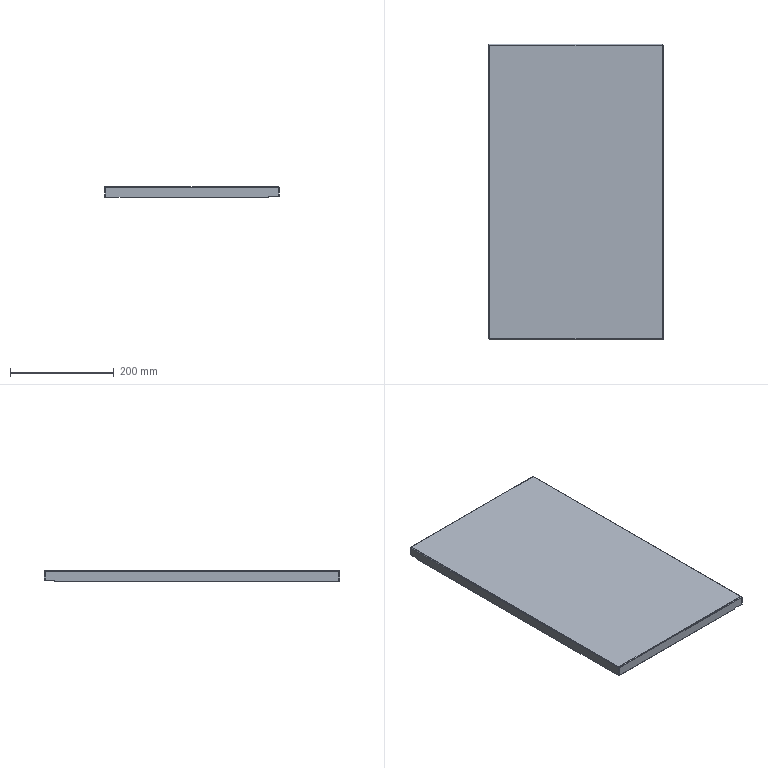Part | SolidWorks | features BaseBody 1 | 1 solid | 44 faces | box 336 x 570 x 20 mm | volume 267174 mm3 | plane 32 | cylinder 8 | spline 4 | commonest cylinder face diameters 1 x4 3.4 x4
STEP:
#1=CARTESIAN_POINT('',(-168.,265.3,-20.));
#2=VERTEX_POINT('',#1);
#3=CARTESIAN_POINT('',(-168.,265.3,-18.));
#4=VERTEX_POINT('',#3);
#5=CARTESIAN_POINT('',(-168.,265.3,-20.));
#6=DIRECTION('',(0.,0.,1.));
#7=VECTOR('',#6,1000.);
#8=LINE('',#5,#7);
#9=EDGE_CURVE('',#2,#4,#8,.T.);
#10=ORIENTED_EDGE('',*,*,#9,.T.);
#11=CARTESIAN_POINT('',(-166.8,265.3,-18.));
#12=VERTEX_POINT('',#11);
#13=CARTESIAN_POINT('',(-166.8,265.3,-18.));
#14=DIRECTION('',(-1.,0.,0.));
#15=VECTOR('',#14,1000.);
#16=LINE('',#13,#15);
#17=EDGE_CURVE('',#12,#4,#16,.T.);
#18=ORIENTED_EDGE('',*,*,#17,.F.);
#19=CARTESIAN_POINT('',(-166.8,265.3,-20.));
#20=VERTEX_POINT('',#19);
#21=CARTESIAN_POINT('',(-166.8,265.3,-20.));
#22=DIRECTION('',(0.,0.,1.));
#23=VECTOR('',#22,1000.);
#24=LINE('',#21,#23);
#25=EDGE_CURVE('',#20,#12,#24,.T.);
#26=ORIENTED_EDGE('',*,*,#25,.F.);
#27=CARTESIAN_POINT('',(-166.8,265.3,-20.));
#28=DIRECTION('',(-1.,0.,0.));
#29=VECTOR('',#28,1000.);
#30=LINE('',#27,#29);
#31=EDGE_CURVE('',#20,#2,#30,.T.);
#32=ORIENTED_EDGE('',*,*,#31,.T.);
#33=EDGE_LOOP('',(#10,#18,#26,#32));
#34=FACE_OUTER_BOUND('',#33,.T.);
#35=CARTESIAN_POINT('',(-166.8,265.3,-20.));
#36=DIRECTION('',(0.,-1.,0.));
#37=DIRECTION('',(0.,0.,-1.));
#38=AXIS2_PLACEMENT_3D('',#35,#36,#37);
#39=PLANE('',#38);
#40=ADVANCED_FACE('',(#34),#39,.F.);
#41=CARTESIAN_POINT('',(-168.,283.3,-18.));
#42=VERTEX_POINT('',#41);
#43=CARTESIAN_POINT('',(-168.,283.3,-18.));
#44=DIRECTION('',(0.,1.,0.));
#45=VECTOR('',#44,1000.);
#46=LINE('',#43,#45);
#47=EDGE_CURVE('',#4,#42,#46,.T.);
#48=ORIENTED_EDGE('',*,*,#47,.T.);
#49=CARTESIAN_POINT('',(-166.8,283.3,-18.));
#50=VERTEX_POINT('',#49);
#51=CARTESIAN_POINT('',(-166.8,283.3,-18.));
#52=DIRECTION('',(-1.,0.,0.));
#53=VECTOR('',#52,1000.);
#54=LINE('',#51,#53);
#55=EDGE_CURVE('',#50,#42,#54,.T.);
#56=ORIENTED_EDGE('',*,*,#55,.F.);
#57=CARTESIAN_POINT('',(-166.8,283.3,-18.));
#58=DIRECTION('',(0.,1.,0.));
#59=VECTOR('',#58,1000.);
#60=LINE('',#57,#59);
#61=EDGE_CURVE('',#12,#50,#60,.T.);
#62=ORIENTED_EDGE('',*,*,#61,.F.);
#63=ORIENTED_EDGE('',*,*,#17,.T.);
#64=EDGE_LOOP('',(#48,#56,#62,#63));
#65=FACE_OUTER_BOUND('',#64,.T.);
#66=CARTESIAN_POINT('',(-166.8,283.3,-18.));
#67=DIRECTION('',(0.,0.,1.));
#68=DIRECTION('',(1.,0.,0.));
#69=AXIS2_PLACEMENT_3D('',#66,#67,#68);
#70=PLANE('',#69);
#71=ADVANCED_FACE('',(#65),#70,.F.);
#72=CARTESIAN_POINT('',(166.3,-285.,-18.));
#73=VERTEX_POINT('',#72);
#74=CARTESIAN_POINT('',(148.3,-285.,-18.));
#75=VERTEX_POINT('',#74);
#76=CARTESIAN_POINT('',(166.3,-285.,-18.));
#77=DIRECTION('',(-1.,0.,0.));
#78=VECTOR('',#77,1000.);
#79=LINE('',#76,#78);
#80=EDGE_CURVE('',#73,#75,#79,.T.);
#81=ORIENTED_EDGE('',*,*,#80,.T.);
#82=CARTESIAN_POINT('',(148.3,-283.8,-18.));
#83=VERTEX_POINT('',#82);
#84=CARTESIAN_POINT('',(148.3,-283.8,-18.));
#85=DIRECTION('',(0.,-1.,0.));
#86=VECTOR('',#85,1000.);
#87=LINE('',#84,#86);
#88=EDGE_CURVE('',#83,#75,#87,.T.);
#89=ORIENTED_EDGE('',*,*,#88,.F.);
#90=CARTESIAN_POINT('',(166.3,-283.8,-18.));
#91=VERTEX_POINT('',#90);
#92=CARTESIAN_POINT('',(166.3,-283.8,-18.));
#93=DIRECTION('',(-1.,0.,0.));
#94=VECTOR('',#93,1000.);
#95=LINE('',#92,#94);
#96=EDGE_CURVE('',#91,#83,#95,.T.);
#97=ORIENTED_EDGE('',*,*,#96,.F.);
#98=CARTESIAN_POINT('',(166.3,-283.8,-18.));
#99=DIRECTION('',(0.,-1.,0.));
#100=VECTOR('',#99,1000.);
#101=LINE('',#98,#100);
#102=EDGE_CURVE('',#91,#73,#101,.T.);
#103=ORIENTED_EDGE('',*,*,#102,.T.);
#104=EDGE_LOOP('',(#81,#89,#97,#103));
#105=FACE_OUTER_BOUND('',#104,.T.);
#106=CARTESIAN_POINT('',(166.3,-283.8,-18.));
#107=DIRECTION('',(0.,0.,1.));
#108=DIRECTION('',(0.,-1.,0.));
#109=AXIS2_PLACEMENT_3D('',#106,#107,#108);
#110=PLANE('',#109);
#111=ADVANCED_FACE('',(#105),#110,.F.);
#112=CARTESIAN_POINT('',(148.3,-285.,-20.));
#113=VERTEX_POINT('',#112);
#114=CARTESIAN_POINT('',(148.3,-285.,-20.));
#115=DIRECTION('',(0.,0.,-1.));
#116=VECTOR('',#115,1000.);
#117=LINE('',#114,#116);
#118=EDGE_CURVE('',#75,#113,#117,.T.);
#119=ORIENTED_EDGE('',*,*,#118,.T.);
#120=CARTESIAN_POINT('',(148.3,-283.8,-20.));
#121=VERTEX_POINT('',#120);
#122=CARTESIAN_POINT('',(148.3,-283.8,-20.));
#123=DIRECTION('',(0.,-1.,0.));
#124=VECTOR('',#123,1000.);
#125=LINE('',#122,#124);
#126=EDGE_CURVE('',#121,#113,#125,.T.);
#127=ORIENTED_EDGE('',*,*,#126,.F.);
#128=CARTESIAN_POINT('',(148.3,-283.8,-20.));
#129=DIRECTION('',(0.,0.,-1.));
#130=VECTOR('',#129,1000.);
#131=LINE('',#128,#130);
#132=EDGE_CURVE('',#83,#121,#131,.T.);
#133=ORIENTED_EDGE('',*,*,#132,.F.);
#134=ORIENTED_EDGE('',*,*,#88,.T.);
#135=EDGE_LOOP('',(#119,#127,#133,#134));
#136=FACE_OUTER_BOUND('',#135,.T.);
#137=CARTESIAN_POINT('',(148.3,-283.8,-20.));
#138=DIRECTION('',(-1.,0.,0.));
#139=DIRECTION('',(0.,0.,1.));
#140=AXIS2_PLACEMENT_3D('',#137,#138,#139);
#141=PLANE('',#140);
#142=ADVANCED_FACE('',(#136),#141,.F.);
#143=CARTESIAN_POINT('',(-166.093,-285.,-20.));
#144=VERTEX_POINT('',#143);
#145=CARTESIAN_POINT('',(-166.093,-283.8,-20.));
#146=VERTEX_POINT('',#145);
#147=CARTESIAN_POINT('',(-166.093,-285.,-20.));
#148=DIRECTION('',(0.,1.,0.));
#149=VECTOR('',#148,1000.);
#150=LINE('',#147,#149);
#151=EDGE_CURVE('',#144,#146,#150,.T.);
#152=ORIENTED_EDGE('',*,*,#151,.F.);
#153=CARTESIAN_POINT('',(-166.093,-285.,-1.7));
#154=VERTEX_POINT('',#153);
#155=CARTESIAN_POINT('',(-166.093,-285.,0.));
#156=DIRECTION('',(0.,0.,-1.));
#157=VECTOR('',#156,1000.);
#158=LINE('',#155,#157);
#159=EDGE_CURVE('',#154,#144,#158,.T.);
#160=ORIENTED_EDGE('',*,*,#159,.F.);
#161=CARTESIAN_POINT('',(-166.093,-283.8,-1.7));
#162=VERTEX_POINT('',#161);
#163=CARTESIAN_POINT('',(-166.093,-283.8,-1.7));
#164=DIRECTION('',(0.,1.,0.));
#165=VECTOR('',#164,1000.);
#166=LINE('',#163,#165);
#167=EDGE_CURVE('',#154,#162,#166,.T.);
#168=ORIENTED_EDGE('',*,*,#167,.T.);
#169=CARTESIAN_POINT('',(-166.093,-283.8,-1.2));
#170=DIRECTION('',(0.,0.,-1.));
#171=VECTOR('',#170,1000.);
#172=LINE('',#169,#171);
#173=EDGE_CURVE('',#162,#146,#172,.T.);
#174=ORIENTED_EDGE('',*,*,#173,.T.);
#175=EDGE_LOOP('',(#152,#160,#168,#174));
#176=FACE_OUTER_BOUND('',#175,.T.);
#177=CARTESIAN_POINT('',(-166.093,-283.8,-1.2));
#178=DIRECTION('',(1.,0.,0.));
#179=DIRECTION('',(0.,1.,0.));
#180=AXIS2_PLACEMENT_3D('',#177,#178,#179);
#181=PLANE('',#180);
#182=ADVANCED_FACE('',(#176),#181,.F.);
#183=CARTESIAN_POINT('',(166.3,-283.8,-20.));
#184=DIRECTION('',(1.,0.,0.));
#185=VECTOR('',#184,1000.);
#186=LINE('',#183,#185);
#187=EDGE_CURVE('',#146,#121,#186,.T.);
#188=ORIENTED_EDGE('',*,*,#187,.T.);
#189=ORIENTED_EDGE('',*,*,#126,.T.);
#190=CARTESIAN_POINT('',(0.,-285.,-20.));
#191=DIRECTION('',(1.,0.,0.));
#192=VECTOR('',#191,1000.);
#193=LINE('',#190,#192);
#194=EDGE_CURVE('',#144,#113,#193,.T.);
#195=ORIENTED_EDGE('',*,*,#194,.F.);
#196=ORIENTED_EDGE('',*,*,#151,.T.);
#197=EDGE_LOOP('',(#188,#189,#195,#196));
#198=FACE_OUTER_BOUND('',#197,.T.);
#199=CARTESIAN_POINT('',(166.3,-285.,-20.));
#200=DIRECTION('',(0.,0.,1.));
#201=DIRECTION('',(0.,-1.,0.));
#202=AXIS2_PLACEMENT_3D('',#199,#200,#201);
#203=PLANE('',#202);
#204=ADVANCED_FACE('',(#198),#203,.F.);
#205=ORIENTED_EDGE('',*,*,#132,.T.);
#206=ORIENTED_EDGE('',*,*,#187,.F.);
#207=ORIENTED_EDGE('',*,*,#173,.F.);
#208=CARTESIAN_POINT('',(166.3,-283.8,-1.7));
#209=VERTEX_POINT('',#208);
#210=CARTESIAN_POINT('',(166.3,-283.8,-1.7));
#211=DIRECTION('',(-1.,0.,0.));
#212=VECTOR('',#211,1000.);
#213=LINE('',#210,#212);
#214=EDGE_CURVE('',#209,#162,#213,.T.);
#215=ORIENTED_EDGE('',*,*,#214,.F.);
#216=CARTESIAN_POINT('',(166.3,-283.8,-1.2));
#217=DIRECTION('',(0.,0.,1.));
#218=VECTOR('',#217,1000.);
#219=LINE('',#216,#218);
#220=EDGE_CURVE('',#91,#209,#219,.T.);
#221=ORIENTED_EDGE('',*,*,#220,.F.);
#222=ORIENTED_EDGE('',*,*,#96,.T.);
#223=EDGE_LOOP('',(#205,#206,#207,#215,#221,#222));
#224=FACE_OUTER_BOUND('',#223,.T.);
#225=CARTESIAN_POINT('',(0.,-283.8,0.));
#226=DIRECTION('',(0.,1.,0.));
#227=DIRECTION('',(0.,0.,-1.));
#228=AXIS2_PLACEMENT_3D('',#225,#226,#227);
#229=PLANE('',#228);
#230=ADVANCED_FACE('',(#224),#229,.T.);
#231=ORIENTED_EDGE('',*,*,#194,.T.);
#232=ORIENTED_EDGE('',*,*,#118,.F.);
#233=ORIENTED_EDGE('',*,*,#80,.F.);
#234=CARTESIAN_POINT('',(166.3,-285.,-1.7));
#235=VERTEX_POINT('',#234);
#236=CARTESIAN_POINT('',(166.3,-285.,0.));
#237=DIRECTION('',(0.,0.,1.));
#238=VECTOR('',#237,1000.);
#239=LINE('',#236,#238);
#240=EDGE_CURVE('',#73,#235,#239,.T.);
#241=ORIENTED_EDGE('',*,*,#240,.T.);
#242=CARTESIAN_POINT('',(166.3,-285.,-1.7));
#243=DIRECTION('',(1.,0.,0.));
#244=VECTOR('',#243,1000.);
#245=LINE('',#242,#244);
#246=EDGE_CURVE('',#154,#235,#245,.T.);
#247=ORIENTED_EDGE('',*,*,#246,.F.);
#248=ORIENTED_EDGE('',*,*,#159,.T.);
#249=EDGE_LOOP('',(#231,#232,#233,#241,#247,#248));
#250=FACE_OUTER_BOUND('',#249,.T.);
#251=CARTESIAN_POINT('',(0.,-285.,0.));
#252=DIRECTION('',(0.,1.,0.));
#253=DIRECTION('',(0.,0.,-1.));
#254=AXIS2_PLACEMENT_3D('',#251,#252,#253);
#255=PLANE('',#254);
#256=ADVANCED_FACE('',(#250),#255,.F.);
#257=ORIENTED_EDGE('',*,*,#240,.F.);
#258=ORIENTED_EDGE('',*,*,#102,.F.);
#259=ORIENTED_EDGE('',*,*,#220,.T.);
#260=CARTESIAN_POINT('',(166.3,-285.,-1.7));
#261=DIRECTION('',(0.,-1.,0.));
#262=VECTOR('',#261,1000.);
#263=LINE('',#260,#262);
#264=EDGE_CURVE('',#209,#235,#263,.T.);
#265=ORIENTED_EDGE('',*,*,#264,.T.);
#266=EDGE_LOOP('',(#257,#258,#259,#265));
#267=FACE_OUTER_BOUND('',#266,.T.);
#268=CARTESIAN_POINT('',(166.3,-285.,-1.2));
#269=DIRECTION('',(-1.,0.,0.));
#270=DIRECTION('',(0.,1.,0.));
#271=AXIS2_PLACEMENT_3D('',#268,#269,#270);
#272=PLANE('',#271);
#273=ADVANCED_FACE('',(#267),#272,.F.);
#274=CARTESIAN_POINT('',(-166.3,-283.3,-1.2));
#275=VERTEX_POINT('',#274);
#276=CARTESIAN_POINT('',(166.3,-283.3,-1.2));
#277=VERTEX_POINT('',#276);
#278=CARTESIAN_POINT('',(-166.3,-283.3,-1.2));
#279=DIRECTION('',(1.,0.,0.));
#280=VECTOR('',#279,1000.);
#281=LINE('',#278,#280);
#282=EDGE_CURVE('',#275,#277,#281,.T.);
#283=ORIENTED_EDGE('',*,*,#282,.T.);
#284=CARTESIAN_POINT('',(166.3,-283.3,-1.7));
#285=DIRECTION('',(1.,0.,0.));
#286=DIRECTION('',(0.,0.,1.));
#287=AXIS2_PLACEMENT_3D('',#284,#285,#286);
#288=CIRCLE('',#287,0.5);
#289=EDGE_CURVE('',#277,#209,#288,.T.);
#290=ORIENTED_EDGE('',*,*,#289,.T.);
#291=ORIENTED_EDGE('',*,*,#214,.T.);
#292=CARTESIAN_POINT('',(-166.093,-283.8,-1.7));
#293=CARTESIAN_POINT('',(-166.127,-283.8,-1.569));
#294=CARTESIAN_POINT('',(-166.162,-283.746,-1.439));
#295=CARTESIAN_POINT('',(-166.231,-283.561,-1.254));
#296=CARTESIAN_POINT('',(-166.265,-283.431,-1.2));
#297=CARTESIAN_POINT('',(-166.3,-283.3,-1.2));
#298=B_SPLINE_CURVE_WITH_KNOTS('',3,(#292,#293,#294,#295,#296,#297),.UNSPECIFIED.,.F.,.F.,(4,2,4),(0.,0.5,1.),.UNSPECIFIED.);
#299=EDGE_CURVE('',#162,#275,#298,.T.);
#300=ORIENTED_EDGE('',*,*,#299,.T.);
#301=EDGE_LOOP('',(#283,#290,#291,#300));
#302=FACE_OUTER_BOUND('',#301,.T.);
#303=CARTESIAN_POINT('',(-166.3,-283.3,-1.7));
#304=DIRECTION('',(-1.,0.,0.));
#305=DIRECTION('',(0.,-1.,0.));
#306=AXIS2_PLACEMENT_3D('',#303,#304,#305);
#307=CYLINDRICAL_SURFACE('',#306,0.5);
#308=ADVANCED_FACE('',(#302),#307,.F.);
#309=CARTESIAN_POINT('',(-166.3,-283.3,0.));
#310=VERTEX_POINT('',#309);
#311=CARTESIAN_POINT('',(166.3,-283.3,0.));
#312=VERTEX_POINT('',#311);
#313=CARTESIAN_POINT('',(-166.3,-283.3,0.));
#314=DIRECTION('',(1.,0.,0.));
#315=VECTOR('',#314,1000.);
#316=LINE('',#313,#315);
#317=EDGE_CURVE('',#310,#312,#316,.T.);
#318=ORIENTED_EDGE('',*,*,#317,.F.);
#319=CARTESIAN_POINT('',(-166.093,-285.,-1.7));
#320=CARTESIAN_POINT('',(-166.11,-285.,-1.477));
#321=CARTESIAN_POINT('',(-166.127,-284.956,-1.255));
#322=CARTESIAN_POINT('',(-166.162,-284.785,-0.8438));
#323=CARTESIAN_POINT('',(-166.179,-284.659,-0.6553));
#324=CARTESIAN_POINT('',(-166.214,-284.345,-0.3406));
#325=CARTESIAN_POINT('',(-166.231,-284.156,-0.2146));
#326=CARTESIAN_POINT('',(-166.265,-283.745,-0.04425));
#327=CARTESIAN_POINT('',(-166.283,-283.523,0.));
#328=CARTESIAN_POINT('',(-166.3,-283.3,0.));
#329=B_SPLINE_CURVE_WITH_KNOTS('',3,(#319,#320,#321,#322,#323,#324,#325,#326,#327,#328),.UNSPECIFIED.,.F.,.F.,(4,2,2,2,4),(0.,0.25,0.5,0.75,1.),.UNSPECIFIED.);
#330=EDGE_CURVE('',#154,#310,#329,.T.);
#331=ORIENTED_EDGE('',*,*,#330,.F.);
#332=ORIENTED_EDGE('',*,*,#246,.T.);
#333=CARTESIAN_POINT('',(166.3,-284.925,-1.2));
#334=VERTEX_POINT('',#333);
#335=CARTESIAN_POINT('',(166.3,-283.3,-1.7));
#336=DIRECTION('',(1.,0.,0.));
#337=DIRECTION('',(0.,0.,1.));
#338=AXIS2_PLACEMENT_3D('',#335,#336,#337);
#339=CIRCLE('',#338,1.7);
#340=EDGE_CURVE('',#334,#235,#339,.T.);
#341=ORIENTED_EDGE('',*,*,#340,.F.);
#342=CARTESIAN_POINT('',(166.3,-283.3,-1.7));
#343=DIRECTION('',(1.,0.,0.));
#344=DIRECTION('',(0.,0.,1.));
#345=AXIS2_PLACEMENT_3D('',#342,#343,#344);
#346=CIRCLE('',#345,1.7);
#347=EDGE_CURVE('',#312,#334,#346,.T.);
#348=ORIENTED_EDGE('',*,*,#347,.F.);
#349=EDGE_LOOP('',(#318,#331,#332,#341,#348));
#350=FACE_OUTER_BOUND('',#349,.T.);
#351=CARTESIAN_POINT('',(-166.3,-283.3,-1.7));
#352=DIRECTION('',(-1.,0.,0.));
#353=DIRECTION('',(0.,-1.,0.));
#354=AXIS2_PLACEMENT_3D('',#351,#352,#353);
#355=CYLINDRICAL_SURFACE('',#354,1.7);
#356=ADVANCED_FACE('',(#350),#355,.T.);
#357=ORIENTED_EDGE('',*,*,#299,.F.);
#358=ORIENTED_EDGE('',*,*,#167,.F.);
#359=ORIENTED_EDGE('',*,*,#330,.T.);
#360=CARTESIAN_POINT('',(-166.3,-283.3,-1.2));
#361=DIRECTION('',(0.,0.,1.));
#362=VECTOR('',#361,1000.);
#363=LINE('',#360,#362);
#364=EDGE_CURVE('',#275,#310,#363,.T.);
#365=ORIENTED_EDGE('',*,*,#364,.F.);
#366=EDGE_LOOP('',(#357,#358,#359,#365));
#367=FACE_OUTER_BOUND('',#366,.T.);
#368=CARTESIAN_POINT('',(-166.093,-285.012,-1.7));
#369=CARTESIAN_POINT('',(-166.11,-285.012,-1.476));
#370=CARTESIAN_POINT('',(-166.127,-284.967,-1.252));
#371=CARTESIAN_POINT('',(-166.162,-284.796,-0.8378));
#372=CARTESIAN_POINT('',(-166.179,-284.669,-0.6479));
#373=CARTESIAN_POINT('',(-166.214,-284.352,-0.331));
#374=CARTESIAN_POINT('',(-166.231,-284.162,-0.2041));
#375=CARTESIAN_POINT('',(-166.265,-283.748,-0.03256));
#376=CARTESIAN_POINT('',(-166.283,-283.524,0.012));
#377=CARTESIAN_POINT('',(-166.3,-283.3,0.012));
#378=CARTESIAN_POINT('',(-166.093,-285.,-1.7));
#379=CARTESIAN_POINT('',(-166.11,-285.,-1.477));
#380=CARTESIAN_POINT('',(-166.127,-284.956,-1.255));
#381=CARTESIAN_POINT('',(-166.162,-284.785,-0.8438));
#382=CARTESIAN_POINT('',(-166.179,-284.659,-0.6553));
#383=CARTESIAN_POINT('',(-166.214,-284.345,-0.3406));
#384=CARTESIAN_POINT('',(-166.231,-284.156,-0.2146));
#385=CARTESIAN_POINT('',(-166.265,-283.745,-0.04425));
#386=CARTESIAN_POINT('',(-166.283,-283.523,0.));
#387=CARTESIAN_POINT('',(-166.3,-283.3,0.));
#388=CARTESIAN_POINT('',(-166.093,-283.8,-1.7));
#389=CARTESIAN_POINT('',(-166.11,-283.8,-1.635));
#390=CARTESIAN_POINT('',(-166.127,-283.787,-1.569));
#391=CARTESIAN_POINT('',(-166.162,-283.737,-1.448));
#392=CARTESIAN_POINT('',(-166.179,-283.7,-1.393));
#393=CARTESIAN_POINT('',(-166.214,-283.607,-1.3));
#394=CARTESIAN_POINT('',(-166.231,-283.552,-1.263));
#395=CARTESIAN_POINT('',(-166.265,-283.431,-1.213));
#396=CARTESIAN_POINT('',(-166.283,-283.365,-1.2));
#397=CARTESIAN_POINT('',(-166.3,-283.3,-1.2));
#398=CARTESIAN_POINT('',(-166.093,-283.788,-1.7));
#399=CARTESIAN_POINT('',(-166.11,-283.788,-1.636));
#400=CARTESIAN_POINT('',(-166.127,-283.775,-1.572));
#401=CARTESIAN_POINT('',(-166.162,-283.726,-1.454));
#402=CARTESIAN_POINT('',(-166.179,-283.69,-1.4));
#403=CARTESIAN_POINT('',(-166.214,-283.6,-1.31));
#404=CARTESIAN_POINT('',(-166.231,-283.546,-1.274));
#405=CARTESIAN_POINT('',(-166.265,-283.428,-1.225));
#406=CARTESIAN_POINT('',(-166.283,-283.364,-1.212));
#407=CARTESIAN_POINT('',(-166.3,-283.3,-1.212));
#408=B_SPLINE_SURFACE_WITH_KNOTS('',1,3,((#368,#369,#370,#371,#372,#373,#374,#375,#376,#377),(#378,#379,#380,#381,#382,#383,#384,#385,#386,#387),(#388,#389,#390,#391,#392,#393,#394,#395,#396,#397),(#398,#399,#400,#401,#402,#403,#404,#405,#406,#407)),.UNSPECIFIED.,.F.,.F.,.F.,(2,1,1,2),(4,2,2,2,4),(-0.01,0.,1.,1.01),(0.,0.25,0.5,0.75,1.),.UNSPECIFIED.);
#409=ADVANCED_FACE('',(#367),#408,.F.);
#410=CARTESIAN_POINT('',(166.3,-285.,-1.2));
#411=DIRECTION('',(0.,1.,0.));
#412=VECTOR('',#411,1000.);
#413=LINE('',#410,#412);
#414=EDGE_CURVE('',#334,#277,#413,.T.);
#415=ORIENTED_EDGE('',*,*,#414,.F.);
#416=ORIENTED_EDGE('',*,*,#340,.T.);
#417=ORIENTED_EDGE('',*,*,#264,.F.);
#418=ORIENTED_EDGE('',*,*,#289,.F.);
#419=EDGE_LOOP('',(#415,#416,#417,#418));
#420=FACE_OUTER_BOUND('',#419,.T.);
#421=CARTESIAN_POINT('',(166.3,-283.3,-1.7));
#422=DIRECTION('',(1.,0.,0.));
#423=DIRECTION('',(0.,1.,0.));
#424=AXIS2_PLACEMENT_3D('',#421,#422,#423);
#425=PLANE('',#424);
#426=ADVANCED_FACE('',(#420),#425,.T.);
#427=CARTESIAN_POINT('',(-166.8,283.3,-1.7));
#428=VERTEX_POINT('',#427);
#429=CARTESIAN_POINT('',(-166.8,283.3,-20.));
#430=DIRECTION('',(0.,0.,-1.));
#431=VECTOR('',#430,1000.);
#432=LINE('',#429,#431);
#433=EDGE_CURVE('',#428,#50,#432,.T.);
#434=ORIENTED_EDGE('',*,*,#433,.T.);
#435=ORIENTED_EDGE('',*,*,#55,.T.);
#436=CARTESIAN_POINT('',(-168.,283.3,-1.7));
#437=VERTEX_POINT('',#436);
#438=CARTESIAN_POINT('',(-168.,283.3,0.));
#439=DIRECTION('',(0.,0.,-1.));
#440=VECTOR('',#439,1000.);
#441=LINE('',#438,#440);
#442=EDGE_CURVE('',#437,#42,#441,.T.);
#443=ORIENTED_EDGE('',*,*,#442,.F.);
#444=CARTESIAN_POINT('',(-166.8,283.3,-1.7));
#445=DIRECTION('',(-1.,0.,0.));
#446=VECTOR('',#445,1000.);
#447=LINE('',#444,#446);
#448=EDGE_CURVE('',#428,#437,#447,.T.);
#449=ORIENTED_EDGE('',*,*,#448,.F.);
#450=EDGE_LOOP('',(#434,#435,#443,#449));
#451=FACE_OUTER_BOUND('',#450,.T.);
#452=CARTESIAN_POINT('',(-168.,283.3,-20.));
#453=DIRECTION('',(0.,-1.,0.));
#454=DIRECTION('',(0.,0.,-1.));
#455=AXIS2_PLACEMENT_3D('',#452,#453,#454);
#456=PLANE('',#455);
#457=ADVANCED_FACE('',(#451),#456,.F.);
#458=CARTESIAN_POINT('',(-168.,-283.093,-20.));
#459=VERTEX_POINT('',#458);
#460=CARTESIAN_POINT('',(-168.,0.,-20.));
#461=DIRECTION('',(0.,-1.,0.));
#462=VECTOR('',#461,1000.);
#463=LINE('',#460,#462);
#464=EDGE_CURVE('',#2,#459,#463,.T.);
#465=ORIENTED_EDGE('',*,*,#464,.F.);
#466=ORIENTED_EDGE('',*,*,#31,.F.);
#467=CARTESIAN_POINT('',(-166.8,-283.093,-20.));
#468=VERTEX_POINT('',#467);
#469=CARTESIAN_POINT('',(-166.8,-285.,-20.));
#470=DIRECTION('',(0.,-1.,0.));
#471=VECTOR('',#470,1000.);
#472=LINE('',#469,#471);
#473=EDGE_CURVE('',#20,#468,#472,.T.);
#474=ORIENTED_EDGE('',*,*,#473,.T.);
#475=CARTESIAN_POINT('',(-166.8,-283.093,-20.));
#476=DIRECTION('',(1.,0.,0.));
#477=VECTOR('',#476,1000.);
#478=LINE('',#475,#477);
#479=EDGE_CURVE('',#459,#468,#478,.T.);
#480=ORIENTED_EDGE('',*,*,#479,.F.);
#481=EDGE_LOOP('',(#465,#466,#474,#480));
#482=FACE_OUTER_BOUND('',#481,.T.);
#483=CARTESIAN_POINT('',(-168.,-285.,-20.));
#484=DIRECTION('',(0.,0.,1.));
#485=DIRECTION('',(1.,0.,0.));
#486=AXIS2_PLACEMENT_3D('',#483,#484,#485);
#487=PLANE('',#486);
#488=ADVANCED_FACE('',(#482),#487,.F.);
#489=ORIENTED_EDGE('',*,*,#61,.T.);
#490=ORIENTED_EDGE('',*,*,#433,.F.);
#491=CARTESIAN_POINT('',(-166.8,-283.093,-1.7));
#492=VERTEX_POINT('',#491);
#493=CARTESIAN_POINT('',(-166.8,-285.,-1.7));
#494=DIRECTION('',(0.,1.,0.));
#495=VECTOR('',#494,1000.);
#496=LINE('',#493,#495);
#497=EDGE_CURVE('',#492,#428,#496,.T.);
#498=ORIENTED_EDGE('',*,*,#497,.F.);
#499=CARTESIAN_POINT('',(-166.8,-283.093,0.));
#500=DIRECTION('',(0.,0.,-1.));
#501=VECTOR('',#500,1000.);
#502=LINE('',#499,#501);
#503=EDGE_CURVE('',#492,#468,#502,.T.);
#504=ORIENTED_EDGE('',*,*,#503,.T.);
#505=ORIENTED_EDGE('',*,*,#473,.F.);
#506=ORIENTED_EDGE('',*,*,#25,.T.);
#507=EDGE_LOOP('',(#489,#490,#498,#504,#505,#506));
#508=FACE_OUTER_BOUND('',#507,.T.);
#509=CARTESIAN_POINT('',(-166.8,0.,0.));
#510=DIRECTION('',(1.,0.,0.));
#511=DIRECTION('',(0.,0.,-1.));
#512=AXIS2_PLACEMENT_3D('',#509,#510,#511);
#513=PLANE('',#512);
#514=ADVANCED_FACE('',(#508),#513,.T.);
#515=ORIENTED_EDGE('',*,*,#442,.T.);
#516=ORIENTED_EDGE('',*,*,#47,.F.);
#517=ORIENTED_EDGE('',*,*,#9,.F.);
#518=ORIENTED_EDGE('',*,*,#464,.T.);
#519=CARTESIAN_POINT('',(-168.,-283.093,-1.7));
#520=VERTEX_POINT('',#519);
#521=CARTESIAN_POINT('',(-168.,-283.093,-1.2));
#522=DIRECTION('',(0.,0.,-1.));
#523=VECTOR('',#522,1000.);
#524=LINE('',#521,#523);
#525=EDGE_CURVE('',#520,#459,#524,.T.);
#526=ORIENTED_EDGE('',*,*,#525,.F.);
#527=CARTESIAN_POINT('',(-168.,-285.,-1.7));
#528=DIRECTION('',(0.,-1.,0.));
#529=VECTOR('',#528,1000.);
#530=LINE('',#527,#529);
#531=EDGE_CURVE('',#437,#520,#530,.T.);
#532=ORIENTED_EDGE('',*,*,#531,.F.);
#533=EDGE_LOOP('',(#515,#516,#517,#518,#526,#532));
#534=FACE_OUTER_BOUND('',#533,.T.);
#535=CARTESIAN_POINT('',(-168.,0.,0.));
#536=DIRECTION('',(1.,0.,0.));
#537=DIRECTION('',(0.,0.,-1.));
#538=AXIS2_PLACEMENT_3D('',#535,#536,#537);
#539=PLANE('',#538);
#540=ADVANCED_FACE('',(#534),#539,.F.);
#541=ORIENTED_EDGE('',*,*,#525,.T.);
#542=ORIENTED_EDGE('',*,*,#479,.T.);
#543=ORIENTED_EDGE('',*,*,#503,.F.);
#544=CARTESIAN_POINT('',(-166.8,-283.093,-1.7));
#545=DIRECTION('',(1.,0.,0.));
#546=VECTOR('',#545,1000.);
#547=LINE('',#544,#546);
#548=EDGE_CURVE('',#520,#492,#547,.T.);
#549=ORIENTED_EDGE('',*,*,#548,.F.);
#550=EDGE_LOOP('',(#541,#542,#543,#549));
#551=FACE_OUTER_BOUND('',#550,.T.);
#552=CARTESIAN_POINT('',(-166.8,-283.093,-1.2));
#553=DIRECTION('',(0.,-1.,0.));
#554=DIRECTION('',(0.,0.,-1.));
#555=AXIS2_PLACEMENT_3D('',#552,#553,#554);
#556=PLANE('',#555);
#557=ADVANCED_FACE('',(#551),#556,.T.);
#558=CARTESIAN_POINT('',(-166.3,283.3,-1.2));
#559=VERTEX_POINT('',#558);
#560=CARTESIAN_POINT('',(-166.3,283.3,-1.2));
#561=DIRECTION('',(0.,-1.,0.));
#562=VECTOR('',#561,1000.);
#563=LINE('',#560,#562);
#564=EDGE_CURVE('',#559,#275,#563,.T.);
#565=ORIENTED_EDGE('',*,*,#564,.T.);
#566=CARTESIAN_POINT('',(-166.3,-283.3,-1.2));
#567=CARTESIAN_POINT('',(-166.431,-283.265,-1.2));
#568=CARTESIAN_POINT('',(-166.561,-283.231,-1.254));
#569=CARTESIAN_POINT('',(-166.746,-283.162,-1.439));
#570=CARTESIAN_POINT('',(-166.8,-283.127,-1.569));
#571=CARTESIAN_POINT('',(-166.8,-283.093,-1.7));
#572=B_SPLINE_CURVE_WITH_KNOTS('',3,(#566,#567,#568,#569,#570,#571),.UNSPECIFIED.,.F.,.F.,(4,2,4),(0.,0.5,1.),.UNSPECIFIED.);
#573=EDGE_CURVE('',#275,#492,#572,.T.);
#574=ORIENTED_EDGE('',*,*,#573,.T.);
#575=ORIENTED_EDGE('',*,*,#497,.T.);
#576=CARTESIAN_POINT('',(-166.3,283.3,-1.7));
#577=DIRECTION('',(0.,1.,0.));
#578=DIRECTION('',(0.,0.,1.));
#579=AXIS2_PLACEMENT_3D('',#576,#577,#578);
#580=CIRCLE('',#579,0.5);
#581=EDGE_CURVE('',#428,#559,#580,.T.);
#582=ORIENTED_EDGE('',*,*,#581,.T.);
#583=EDGE_LOOP('',(#565,#574,#575,#582));
#584=FACE_OUTER_BOUND('',#583,.T.);
#585=CARTESIAN_POINT('',(-166.3,283.3,-1.7));
#586=DIRECTION('',(0.,1.,0.));
#587=DIRECTION('',(-1.,0.,0.));
#588=AXIS2_PLACEMENT_3D('',#585,#586,#587);
#589=CYLINDRICAL_SURFACE('',#588,0.5);
#590=ADVANCED_FACE('',(#584),#589,.F.);
#591=CARTESIAN_POINT('',(-166.3,283.3,0.));
#592=VERTEX_POINT('',#591);
#593=CARTESIAN_POINT('',(-166.3,283.3,0.));
#594=DIRECTION('',(0.,-1.,0.));
#595=VECTOR('',#594,1000.);
#596=LINE('',#593,#595);
#597=EDGE_CURVE('',#592,#310,#596,.T.);
#598=ORIENTED_EDGE('',*,*,#597,.F.);
#599=CARTESIAN_POINT('',(-167.925,283.3,-1.2));
#600=VERTEX_POINT('',#599);
#601=CARTESIAN_POINT('',(-166.3,283.3,-1.7));
#602=DIRECTION('',(0.,1.,0.));
#603=DIRECTION('',(0.,0.,1.));
#604=AXIS2_PLACEMENT_3D('',#601,#602,#603);
#605=CIRCLE('',#604,1.7);
#606=EDGE_CURVE('',#600,#592,#605,.T.);
#607=ORIENTED_EDGE('',*,*,#606,.F.);
#608=CARTESIAN_POINT('',(-166.3,283.3,-1.7));
#609=DIRECTION('',(0.,1.,0.));
#610=DIRECTION('',(0.,0.,1.));
#611=AXIS2_PLACEMENT_3D('',#608,#609,#610);
#612=CIRCLE('',#611,1.7);
#613=EDGE_CURVE('',#437,#600,#612,.T.);
#614=ORIENTED_EDGE('',*,*,#613,.F.);
#615=ORIENTED_EDGE('',*,*,#531,.T.);
#616=CARTESIAN_POINT('',(-166.3,-283.3,0.));
#617=CARTESIAN_POINT('',(-166.523,-283.283,0.));
#618=CARTESIAN_POINT('',(-166.745,-283.265,-0.04425));
#619=CARTESIAN_POINT('',(-167.156,-283.231,-0.2146));
#620=CARTESIAN_POINT('',(-167.345,-283.214,-0.3406));
#621=CARTESIAN_POINT('',(-167.659,-283.179,-0.6553));
#622=CARTESIAN_POINT('',(-167.785,-283.162,-0.8438));
#623=CARTESIAN_POINT('',(-167.956,-283.127,-1.255));
#624=CARTESIAN_POINT('',(-168.,-283.11,-1.477));
#625=CARTESIAN_POINT('',(-168.,-283.093,-1.7));
#626=B_SPLINE_CURVE_WITH_KNOTS('',3,(#616,#617,#618,#619,#620,#621,#622,#623,#624,#625),.UNSPECIFIED.,.F.,.F.,(4,2,2,2,4),(0.,0.25,0.5,0.75,1.),.UNSPECIFIED.);
#627=EDGE_CURVE('',#310,#520,#626,.T.);
#628=ORIENTED_EDGE('',*,*,#627,.F.);
#629=EDGE_LOOP('',(#598,#607,#614,#615,#628));
#630=FACE_OUTER_BOUND('',#629,.T.);
#631=CARTESIAN_POINT('',(-166.3,283.3,-1.7));
#632=DIRECTION('',(0.,1.,0.));
#633=DIRECTION('',(-1.,0.,0.));
#634=AXIS2_PLACEMENT_3D('',#631,#632,#633);
#635=CYLINDRICAL_SURFACE('',#634,1.7);
#636=ADVANCED_FACE('',(#630),#635,.T.);
#637=ORIENTED_EDGE('',*,*,#613,.T.);
#638=CARTESIAN_POINT('',(-168.,283.3,-1.2));
#639=DIRECTION('',(1.,0.,0.));
#640=VECTOR('',#639,1000.);
#641=LINE('',#638,#640);
#642=EDGE_CURVE('',#600,#559,#641,.T.);
#643=ORIENTED_EDGE('',*,*,#642,.T.);
#644=ORIENTED_EDGE('',*,*,#581,.F.);
#645=ORIENTED_EDGE('',*,*,#448,.T.);
#646=EDGE_LOOP('',(#637,#643,#644,#645));
#647=FACE_OUTER_BOUND('',#646,.T.);
#648=CARTESIAN_POINT('',(-166.3,283.3,-1.7));
#649=DIRECTION('',(0.,-1.,0.));
#650=DIRECTION('',(0.,0.,-1.));
#651=AXIS2_PLACEMENT_3D('',#648,#649,#650);
#652=PLANE('',#651);
#653=ADVANCED_FACE('',(#647),#652,.F.);
#654=ORIENTED_EDGE('',*,*,#548,.T.);
#655=ORIENTED_EDGE('',*,*,#573,.F.);
#656=ORIENTED_EDGE('',*,*,#364,.T.);
#657=ORIENTED_EDGE('',*,*,#627,.T.);
#658=EDGE_LOOP('',(#654,#655,#656,#657));
#659=FACE_OUTER_BOUND('',#658,.T.);
#660=CARTESIAN_POINT('',(-166.3,-283.3,0.012));
#661=CARTESIAN_POINT('',(-166.524,-283.283,0.012));
#662=CARTESIAN_POINT('',(-166.748,-283.265,-0.03256));
#663=CARTESIAN_POINT('',(-167.162,-283.231,-0.2041));
#664=CARTESIAN_POINT('',(-167.352,-283.214,-0.331));
#665=CARTESIAN_POINT('',(-167.669,-283.179,-0.6479));
#666=CARTESIAN_POINT('',(-167.796,-283.162,-0.8378));
#667=CARTESIAN_POINT('',(-167.967,-283.127,-1.252));
#668=CARTESIAN_POINT('',(-168.012,-283.11,-1.476));
#669=CARTESIAN_POINT('',(-168.012,-283.093,-1.7));
#670=CARTESIAN_POINT('',(-166.3,-283.3,0.));
#671=CARTESIAN_POINT('',(-166.523,-283.283,0.));
#672=CARTESIAN_POINT('',(-166.745,-283.265,-0.04425));
#673=CARTESIAN_POINT('',(-167.156,-283.231,-0.2146));
#674=CARTESIAN_POINT('',(-167.345,-283.214,-0.3406));
#675=CARTESIAN_POINT('',(-167.659,-283.179,-0.6553));
#676=CARTESIAN_POINT('',(-167.785,-283.162,-0.8438));
#677=CARTESIAN_POINT('',(-167.956,-283.127,-1.255));
#678=CARTESIAN_POINT('',(-168.,-283.11,-1.477));
#679=CARTESIAN_POINT('',(-168.,-283.093,-1.7));
#680=CARTESIAN_POINT('',(-166.3,-283.3,-1.2));
#681=CARTESIAN_POINT('',(-166.365,-283.283,-1.2));
#682=CARTESIAN_POINT('',(-166.431,-283.265,-1.213));
#683=CARTESIAN_POINT('',(-166.552,-283.231,-1.263));
#684=CARTESIAN_POINT('',(-166.607,-283.214,-1.3));
#685=CARTESIAN_POINT('',(-166.7,-283.179,-1.393));
#686=CARTESIAN_POINT('',(-166.737,-283.162,-1.448));
#687=CARTESIAN_POINT('',(-166.787,-283.127,-1.569));
#688=CARTESIAN_POINT('',(-166.8,-283.11,-1.635));
#689=CARTESIAN_POINT('',(-166.8,-283.093,-1.7));
#690=CARTESIAN_POINT('',(-166.3,-283.3,-1.212));
#691=CARTESIAN_POINT('',(-166.364,-283.283,-1.212));
#692=CARTESIAN_POINT('',(-166.428,-283.265,-1.225));
#693=CARTESIAN_POINT('',(-166.546,-283.231,-1.274));
#694=CARTESIAN_POINT('',(-166.6,-283.214,-1.31));
#695=CARTESIAN_POINT('',(-166.69,-283.179,-1.4));
#696=CARTESIAN_POINT('',(-166.726,-283.162,-1.454));
#697=CARTESIAN_POINT('',(-166.775,-283.127,-1.572));
#698=CARTESIAN_POINT('',(-166.788,-283.11,-1.636));
#699=CARTESIAN_POINT('',(-166.788,-283.093,-1.7));
#700=B_SPLINE_SURFACE_WITH_KNOTS('',1,3,((#660,#661,#662,#663,#664,#665,#666,#667,#668,#669),(#670,#671,#672,#673,#674,#675,#676,#677,#678,#679),(#680,#681,#682,#683,#684,#685,#686,#687,#688,#689),(#690,#691,#692,#693,#694,#695,#696,#697,#698,#699)),.UNSPECIFIED.,.F.,.F.,.F.,(2,1,1,2),(4,2,2,2,4),(-0.01,0.,1.,1.01),(0.,0.25,0.5,0.75,1.),.UNSPECIFIED.);
#701=ADVANCED_FACE('',(#659),#700,.F.);
#702=CARTESIAN_POINT('',(166.093,285.,-18.));
#703=VERTEX_POINT('',#702);
#704=CARTESIAN_POINT('',(166.093,283.8,-18.));
#705=VERTEX_POINT('',#704);
#706=CARTESIAN_POINT('',(166.093,285.,-18.));
#707=DIRECTION('',(0.,-1.,0.));
#708=VECTOR('',#707,1000.);
#709=LINE('',#706,#708);
#710=EDGE_CURVE('',#703,#705,#709,.T.);
#711=ORIENTED_EDGE('',*,*,#710,.F.);
#712=CARTESIAN_POINT('',(166.093,285.,-1.7));
#713=VERTEX_POINT('',#712);
#714=CARTESIAN_POINT('',(166.093,285.,0.));
#715=DIRECTION('',(0.,0.,-1.));
#716=VECTOR('',#715,1000.);
#717=LINE('',#714,#716);
#718=EDGE_CURVE('',#713,#703,#717,.T.);
#719=ORIENTED_EDGE('',*,*,#718,.F.);
#720=CARTESIAN_POINT('',(166.093,283.8,-1.7));
#721=VERTEX_POINT('',#720);
#722=CARTESIAN_POINT('',(166.093,283.8,-1.7));
#723=DIRECTION('',(0.,-1.,0.));
#724=VECTOR('',#723,1000.);
#725=LINE('',#722,#724);
#726=EDGE_CURVE('',#713,#721,#725,.T.);
#727=ORIENTED_EDGE('',*,*,#726,.T.);
#728=CARTESIAN_POINT('',(166.093,283.8,-1.2));
#729=DIRECTION('',(0.,0.,-1.));
#730=VECTOR('',#729,1000.);
#731=LINE('',#728,#730);
#732=EDGE_CURVE('',#721,#705,#731,.T.);
#733=ORIENTED_EDGE('',*,*,#732,.T.);
#734=EDGE_LOOP('',(#711,#719,#727,#733));
#735=FACE_OUTER_BOUND('',#734,.T.);
#736=CARTESIAN_POINT('',(166.093,283.8,-1.2));
#737=DIRECTION('',(-1.,0.,0.));
#738=DIRECTION('',(0.,0.,1.));
#739=AXIS2_PLACEMENT_3D('',#736,#737,#738);
#740=PLANE('',#739);
#741=ADVANCED_FACE('',(#735),#740,.F.);
#742=CARTESIAN_POINT('',(-168.,285.,-18.));
#743=VERTEX_POINT('',#742);
#744=CARTESIAN_POINT('',(0.,285.,-18.));
#745=DIRECTION('',(-1.,0.,0.));
#746=VECTOR('',#745,1000.);
#747=LINE('',#744,#746);
#748=EDGE_CURVE('',#703,#743,#747,.T.);
#749=ORIENTED_EDGE('',*,*,#748,.F.);
#750=ORIENTED_EDGE('',*,*,#710,.T.);
#751=CARTESIAN_POINT('',(-168.,283.8,-18.));
#752=VERTEX_POINT('',#751);
#753=CARTESIAN_POINT('',(-168.,283.8,-18.));
#754=DIRECTION('',(-1.,0.,0.));
#755=VECTOR('',#754,1000.);
#756=LINE('',#753,#755);
#757=EDGE_CURVE('',#705,#752,#756,.T.);
#758=ORIENTED_EDGE('',*,*,#757,.T.);
#759=CARTESIAN_POINT('',(-168.,285.,-18.));
#760=DIRECTION('',(0.,-1.,0.));
#761=VECTOR('',#760,1000.);
#762=LINE('',#759,#761);
#763=EDGE_CURVE('',#743,#752,#762,.T.);
#764=ORIENTED_EDGE('',*,*,#763,.F.);
#765=EDGE_LOOP('',(#749,#750,#758,#764));
#766=FACE_OUTER_BOUND('',#765,.T.);
#767=CARTESIAN_POINT('',(-168.,285.,-18.));
#768=DIRECTION('',(0.,0.,1.));
#769=DIRECTION('',(0.,-1.,0.));
#770=AXIS2_PLACEMENT_3D('',#767,#768,#769);
#771=PLANE('',#770);
#772=ADVANCED_FACE('',(#766),#771,.F.);
#773=ORIENTED_EDGE('',*,*,#732,.F.);
#774=CARTESIAN_POINT('',(-168.,283.8,-1.7));
#775=VERTEX_POINT('',#774);
#776=CARTESIAN_POINT('',(-168.,283.8,-1.7));
#777=DIRECTION('',(1.,0.,0.));
#778=VECTOR('',#777,1000.);
#779=LINE('',#776,#778);
#780=EDGE_CURVE('',#775,#721,#779,.T.);
#781=ORIENTED_EDGE('',*,*,#780,.F.);
#782=CARTESIAN_POINT('',(-168.,283.8,-1.2));
#783=DIRECTION('',(0.,0.,1.));
#784=VECTOR('',#783,1000.);
#785=LINE('',#782,#784);
#786=EDGE_CURVE('',#752,#775,#785,.T.);
#787=ORIENTED_EDGE('',*,*,#786,.F.);
#788=ORIENTED_EDGE('',*,*,#757,.F.);
#789=EDGE_LOOP('',(#773,#781,#787,#788));
#790=FACE_OUTER_BOUND('',#789,.T.);
#791=CARTESIAN_POINT('',(0.,283.8,0.));
#792=DIRECTION('',(0.,-1.,0.));
#793=DIRECTION('',(0.,0.,-1.));
#794=AXIS2_PLACEMENT_3D('',#791,#792,#793);
#795=PLANE('',#794);
#796=ADVANCED_FACE('',(#790),#795,.T.);
#797=CARTESIAN_POINT('',(-168.,285.,-1.7));
#798=VERTEX_POINT('',#797);
#799=CARTESIAN_POINT('',(-168.,285.,-1.7));
#800=DIRECTION('',(-1.,0.,0.));
#801=VECTOR('',#800,1000.);
#802=LINE('',#799,#801);
#803=EDGE_CURVE('',#713,#798,#802,.T.);
#804=ORIENTED_EDGE('',*,*,#803,.F.);
#805=ORIENTED_EDGE('',*,*,#718,.T.);
#806=ORIENTED_EDGE('',*,*,#748,.T.);
#807=CARTESIAN_POINT('',(-168.,285.,0.));
#808=DIRECTION('',(0.,0.,1.));
#809=VECTOR('',#808,1000.);
#810=LINE('',#807,#809);
#811=EDGE_CURVE('',#743,#798,#810,.T.);
#812=ORIENTED_EDGE('',*,*,#811,.T.);
#813=EDGE_LOOP('',(#804,#805,#806,#812));
#814=FACE_OUTER_BOUND('',#813,.T.);
#815=CARTESIAN_POINT('',(0.,285.,0.));
#816=DIRECTION('',(0.,-1.,0.));
#817=DIRECTION('',(0.,0.,-1.));
#818=AXIS2_PLACEMENT_3D('',#815,#816,#817);
#819=PLANE('',#818);
#820=ADVANCED_FACE('',(#814),#819,.F.);
#821=CARTESIAN_POINT('',(-168.,285.,-1.7));
#822=DIRECTION('',(0.,1.,0.));
#823=VECTOR('',#822,1000.);
#824=LINE('',#821,#823);
#825=EDGE_CURVE('',#775,#798,#824,.T.);
#826=ORIENTED_EDGE('',*,*,#825,.T.);
#827=ORIENTED_EDGE('',*,*,#811,.F.);
#828=ORIENTED_EDGE('',*,*,#763,.T.);
#829=ORIENTED_EDGE('',*,*,#786,.T.);
#830=EDGE_LOOP('',(#826,#827,#828,#829));
#831=FACE_OUTER_BOUND('',#830,.T.);
#832=CARTESIAN_POINT('',(-168.,285.,-1.2));
#833=DIRECTION('',(1.,0.,0.));
#834=DIRECTION('',(0.,1.,0.));
#835=AXIS2_PLACEMENT_3D('',#832,#833,#834);
#836=PLANE('',#835);
#837=ADVANCED_FACE('',(#831),#836,.F.);
#838=CARTESIAN_POINT('',(166.3,283.3,-1.2));
#839=VERTEX_POINT('',#838);
#840=CARTESIAN_POINT('',(166.3,283.3,-1.2));
#841=DIRECTION('',(-1.,0.,0.));
#842=VECTOR('',#841,1000.);
#843=LINE('',#840,#842);
#844=EDGE_CURVE('',#839,#559,#843,.T.);
#845=ORIENTED_EDGE('',*,*,#844,.T.);
#846=ORIENTED_EDGE('',*,*,#642,.F.);
#847=CARTESIAN_POINT('',(-168.,283.3,-1.2));
#848=VERTEX_POINT('',#847);
#849=CARTESIAN_POINT('',(-168.,283.3,-1.2));
#850=DIRECTION('',(1.,0.,0.));
#851=VECTOR('',#850,1000.);
#852=LINE('',#849,#851);
#853=EDGE_CURVE('',#848,#600,#852,.T.);
#854=ORIENTED_EDGE('',*,*,#853,.F.);
#855=CARTESIAN_POINT('',(-168.,283.3,-1.7));
#856=DIRECTION('',(-1.,0.,0.));
#857=DIRECTION('',(0.,0.,-1.));
#858=AXIS2_PLACEMENT_3D('',#855,#856,#857);
#859=CIRCLE('',#858,0.5);
#860=EDGE_CURVE('',#848,#775,#859,.T.);
#861=ORIENTED_EDGE('',*,*,#860,.T.);
#862=ORIENTED_EDGE('',*,*,#780,.T.);
#863=CARTESIAN_POINT('',(166.093,283.8,-1.7));
#864=CARTESIAN_POINT('',(166.127,283.8,-1.569));
#865=CARTESIAN_POINT('',(166.162,283.746,-1.439));
#866=CARTESIAN_POINT('',(166.231,283.561,-1.254));
#867=CARTESIAN_POINT('',(166.265,283.431,-1.2));
#868=CARTESIAN_POINT('',(166.3,283.3,-1.2));
#869=B_SPLINE_CURVE_WITH_KNOTS('',3,(#863,#864,#865,#866,#867,#868),.UNSPECIFIED.,.F.,.F.,(4,2,4),(0.,0.5,1.),.UNSPECIFIED.);
#870=EDGE_CURVE('',#721,#839,#869,.T.);
#871=ORIENTED_EDGE('',*,*,#870,.T.);
#872=EDGE_LOOP('',(#845,#846,#854,#861,#862,#871));
#873=FACE_OUTER_BOUND('',#872,.T.);
#874=CARTESIAN_POINT('',(166.3,283.3,-1.7));
#875=DIRECTION('',(1.,0.,0.));
#876=DIRECTION('',(0.,1.,0.));
#877=AXIS2_PLACEMENT_3D('',#874,#875,#876);
#878=CYLINDRICAL_SURFACE('',#877,0.5);
#879=ADVANCED_FACE('',(#873),#878,.F.);
#880=CARTESIAN_POINT('',(166.3,283.3,0.));
#881=VERTEX_POINT('',#880);
#882=CARTESIAN_POINT('',(166.3,283.3,0.));
#883=DIRECTION('',(-1.,0.,0.));
#884=VECTOR('',#883,1000.);
#885=LINE('',#882,#884);
#886=EDGE_CURVE('',#881,#592,#885,.T.);
#887=ORIENTED_EDGE('',*,*,#886,.F.);
#888=CARTESIAN_POINT('',(166.093,285.,-1.7));
#889=CARTESIAN_POINT('',(166.11,285.,-1.477));
#890=CARTESIAN_POINT('',(166.127,284.956,-1.255));
#891=CARTESIAN_POINT('',(166.162,284.785,-0.8438));
#892=CARTESIAN_POINT('',(166.179,284.659,-0.6553));
#893=CARTESIAN_POINT('',(166.214,284.345,-0.3406));
#894=CARTESIAN_POINT('',(166.231,284.156,-0.2146));
#895=CARTESIAN_POINT('',(166.265,283.745,-0.04425));
#896=CARTESIAN_POINT('',(166.283,283.523,0.));
#897=CARTESIAN_POINT('',(166.3,283.3,0.));
#898=B_SPLINE_CURVE_WITH_KNOTS('',3,(#888,#889,#890,#891,#892,#893,#894,#895,#896,#897),.UNSPECIFIED.,.F.,.F.,(4,2,2,2,4),(0.,0.25,0.5,0.75,1.),.UNSPECIFIED.);
#899=EDGE_CURVE('',#713,#881,#898,.T.);
#900=ORIENTED_EDGE('',*,*,#899,.F.);
#901=ORIENTED_EDGE('',*,*,#803,.T.);
#902=CARTESIAN_POINT('',(-168.,283.3,0.));
#903=VERTEX_POINT('',#902);
#904=CARTESIAN_POINT('',(-168.,283.3,-1.7));
#905=DIRECTION('',(-1.,0.,0.));
#906=DIRECTION('',(0.,0.,-1.));
#907=AXIS2_PLACEMENT_3D('',#904,#905,#906);
#908=CIRCLE('',#907,1.7);
#909=EDGE_CURVE('',#903,#798,#908,.T.);
#910=ORIENTED_EDGE('',*,*,#909,.F.);
#911=CARTESIAN_POINT('',(166.3,283.3,0.));
#912=DIRECTION('',(1.,0.,0.));
#913=VECTOR('',#912,1000.);
#914=LINE('',#911,#913);
#915=EDGE_CURVE('',#903,#592,#914,.T.);
#916=ORIENTED_EDGE('',*,*,#915,.T.);
#917=EDGE_LOOP('',(#887,#900,#901,#910,#916));
#918=FACE_OUTER_BOUND('',#917,.T.);
#919=CARTESIAN_POINT('',(166.3,283.3,-1.7));
#920=DIRECTION('',(1.,0.,0.));
#921=DIRECTION('',(0.,1.,0.));
#922=AXIS2_PLACEMENT_3D('',#919,#920,#921);
#923=CYLINDRICAL_SURFACE('',#922,1.7);
#924=ADVANCED_FACE('',(#918),#923,.T.);
#925=ORIENTED_EDGE('',*,*,#870,.F.);
#926=ORIENTED_EDGE('',*,*,#726,.F.);
#927=ORIENTED_EDGE('',*,*,#899,.T.);
#928=CARTESIAN_POINT('',(166.3,283.3,-1.2));
#929=DIRECTION('',(0.,0.,1.));
#930=VECTOR('',#929,1000.);
#931=LINE('',#928,#930);
#932=EDGE_CURVE('',#839,#881,#931,.T.);
#933=ORIENTED_EDGE('',*,*,#932,.F.);
#934=EDGE_LOOP('',(#925,#926,#927,#933));
#935=FACE_OUTER_BOUND('',#934,.T.);
#936=CARTESIAN_POINT('',(166.093,285.012,-1.7));
#937=CARTESIAN_POINT('',(166.11,285.012,-1.476));
#938=CARTESIAN_POINT('',(166.127,284.967,-1.252));
#939=CARTESIAN_POINT('',(166.162,284.796,-0.8378));
#940=CARTESIAN_POINT('',(166.179,284.669,-0.6479));
#941=CARTESIAN_POINT('',(166.214,284.352,-0.331));
#942=CARTESIAN_POINT('',(166.231,284.162,-0.2041));
#943=CARTESIAN_POINT('',(166.265,283.748,-0.03256));
#944=CARTESIAN_POINT('',(166.283,283.524,0.012));
#945=CARTESIAN_POINT('',(166.3,283.3,0.012));
#946=CARTESIAN_POINT('',(166.093,285.,-1.7));
#947=CARTESIAN_POINT('',(166.11,285.,-1.477));
#948=CARTESIAN_POINT('',(166.127,284.956,-1.255));
#949=CARTESIAN_POINT('',(166.162,284.785,-0.8438));
#950=CARTESIAN_POINT('',(166.179,284.659,-0.6553));
#951=CARTESIAN_POINT('',(166.214,284.345,-0.3406));
#952=CARTESIAN_POINT('',(166.231,284.156,-0.2146));
#953=CARTESIAN_POINT('',(166.265,283.745,-0.04425));
#954=CARTESIAN_POINT('',(166.283,283.523,0.));
#955=CARTESIAN_POINT('',(166.3,283.3,0.));
#956=CARTESIAN_POINT('',(166.093,283.8,-1.7));
#957=CARTESIAN_POINT('',(166.11,283.8,-1.635));
#958=CARTESIAN_POINT('',(166.127,283.787,-1.569));
#959=CARTESIAN_POINT('',(166.162,283.737,-1.448));
#960=CARTESIAN_POINT('',(166.179,283.7,-1.393));
#961=CARTESIAN_POINT('',(166.214,283.607,-1.3));
#962=CARTESIAN_POINT('',(166.231,283.552,-1.263));
#963=CARTESIAN_POINT('',(166.265,283.431,-1.213));
#964=CARTESIAN_POINT('',(166.283,283.365,-1.2));
#965=CARTESIAN_POINT('',(166.3,283.3,-1.2));
#966=CARTESIAN_POINT('',(166.093,283.788,-1.7));
#967=CARTESIAN_POINT('',(166.11,283.788,-1.636));
#968=CARTESIAN_POINT('',(166.127,283.775,-1.572));
#969=CARTESIAN_POINT('',(166.162,283.726,-1.454));
#970=CARTESIAN_POINT('',(166.179,283.69,-1.4));
#971=CARTESIAN_POINT('',(166.214,283.6,-1.31));
#972=CARTESIAN_POINT('',(166.231,283.546,-1.274));
#973=CARTESIAN_POINT('',(166.265,283.428,-1.225));
#974=CARTESIAN_POINT('',(166.283,283.364,-1.212));
#975=CARTESIAN_POINT('',(166.3,283.3,-1.212));
#976=B_SPLINE_SURFACE_WITH_KNOTS('',1,3,((#936,#937,#938,#939,#940,#941,#942,#943,#944,#945),(#946,#947,#948,#949,#950,#951,#952,#953,#954,#955),(#956,#957,#958,#959,#960,#961,#962,#963,#964,#965),(#966,#967,#968,#969,#970,#971,#972,#973,#974,#975)),.UNSPECIFIED.,.F.,.F.,.F.,(2,1,1,2),(4,2,2,2,4),(-0.01,0.,1.,1.01),(0.,0.25,0.5,0.75,1.),.UNSPECIFIED.);
#977=ADVANCED_FACE('',(#935),#976,.F.);
#978=ORIENTED_EDGE('',*,*,#825,.F.);
#979=ORIENTED_EDGE('',*,*,#860,.F.);
#980=CARTESIAN_POINT('',(-168.,283.3,-1.2));
#981=DIRECTION('',(0.,0.,1.));
#982=VECTOR('',#981,1000.);
#983=LINE('',#980,#982);
#984=EDGE_CURVE('',#848,#903,#983,.T.);
#985=ORIENTED_EDGE('',*,*,#984,.T.);
#986=ORIENTED_EDGE('',*,*,#909,.T.);
#987=EDGE_LOOP('',(#978,#979,#985,#986));
#988=FACE_OUTER_BOUND('',#987,.T.);
#989=CARTESIAN_POINT('',(-168.,283.3,-1.7));
#990=DIRECTION('',(-1.,0.,0.));
#991=DIRECTION('',(0.,0.,1.));
#992=AXIS2_PLACEMENT_3D('',#989,#990,#991);
#993=PLANE('',#992);
#994=ADVANCED_FACE('',(#988),#993,.T.);
#995=CARTESIAN_POINT('',(166.8,-285.,-1.7));
#996=VERTEX_POINT('',#995);
#997=CARTESIAN_POINT('',(168.,-285.,-1.7));
#998=VERTEX_POINT('',#997);
#999=CARTESIAN_POINT('',(166.8,-285.,-1.7));
#1000=DIRECTION('',(1.,0.,0.));
#1001=VECTOR('',#1000,1000.);
#1002=LINE('',#999,#1001);
#1003=EDGE_CURVE('',#996,#998,#1002,.T.);
#1004=ORIENTED_EDGE('',*,*,#1003,.F.);
#1005=CARTESIAN_POINT('',(166.8,-285.,-18.));
#1006=VERTEX_POINT('',#1005);
#1007=CARTESIAN_POINT('',(166.8,-285.,-18.));
#1008=DIRECTION('',(0.,0.,-1.));
#1009=VECTOR('',#1008,1000.);
#1010=LINE('',#1007,#1009);
#1011=EDGE_CURVE('',#996,#1006,#1010,.T.);
#1012=ORIENTED_EDGE('',*,*,#1011,.T.);
#1013=CARTESIAN_POINT('',(168.,-285.,-18.));
#1014=VERTEX_POINT('',#1013);
#1015=CARTESIAN_POINT('',(168.,-285.,-18.));
#1016=DIRECTION('',(-1.,0.,0.));
#1017=VECTOR('',#1016,1000.);
#1018=LINE('',#1015,#1017);
#1019=EDGE_CURVE('',#1014,#1006,#1018,.T.);
#1020=ORIENTED_EDGE('',*,*,#1019,.F.);
#1021=CARTESIAN_POINT('',(168.,-285.,0.));
#1022=DIRECTION('',(0.,0.,-1.));
#1023=VECTOR('',#1022,1000.);
#1024=LINE('',#1021,#1023);
#1025=EDGE_CURVE('',#998,#1014,#1024,.T.);
#1026=ORIENTED_EDGE('',*,*,#1025,.F.);
#1027=EDGE_LOOP('',(#1004,#1012,#1020,#1026));
#1028=FACE_OUTER_BOUND('',#1027,.T.);
#1029=CARTESIAN_POINT('',(168.,-285.,-18.));
#1030=DIRECTION('',(0.,1.,0.));
#1031=DIRECTION('',(0.,0.,-1.));
#1032=AXIS2_PLACEMENT_3D('',#1029,#1030,#1031);
#1033=PLANE('',#1032);
#1034=ADVANCED_FACE('',(#1028),#1033,.F.);
#1035=CARTESIAN_POINT('',(168.,283.093,-18.));
#1036=VERTEX_POINT('',#1035);
#1037=CARTESIAN_POINT('',(166.8,283.093,-18.));
#1038=VERTEX_POINT('',#1037);
#1039=CARTESIAN_POINT('',(166.8,283.093,-18.));
#1040=DIRECTION('',(-1.,0.,0.));
#1041=VECTOR('',#1040,1000.);
#1042=LINE('',#1039,#1041);
#1043=EDGE_CURVE('',#1036,#1038,#1042,.T.);
#1044=ORIENTED_EDGE('',*,*,#1043,.F.);
#1045=CARTESIAN_POINT('',(168.,0.,-18.));
#1046=DIRECTION('',(0.,1.,0.));
#1047=VECTOR('',#1046,1000.);
#1048=LINE('',#1045,#1047);
#1049=EDGE_CURVE('',#1014,#1036,#1048,.T.);
#1050=ORIENTED_EDGE('',*,*,#1049,.F.);
#1051=ORIENTED_EDGE('',*,*,#1019,.T.);
#1052=CARTESIAN_POINT('',(166.8,285.,-18.));
#1053=DIRECTION('',(0.,1.,0.));
#1054=VECTOR('',#1053,1000.);
#1055=LINE('',#1052,#1054);
#1056=EDGE_CURVE('',#1006,#1038,#1055,.T.);
#1057=ORIENTED_EDGE('',*,*,#1056,.T.);
#1058=EDGE_LOOP('',(#1044,#1050,#1051,#1057));
#1059=FACE_OUTER_BOUND('',#1058,.T.);
#1060=CARTESIAN_POINT('',(168.,285.,-18.));
#1061=DIRECTION('',(0.,0.,1.));
#1062=DIRECTION('',(1.,0.,0.));
#1063=AXIS2_PLACEMENT_3D('',#1060,#1061,#1062);
#1064=PLANE('',#1063);
#1065=ADVANCED_FACE('',(#1059),#1064,.F.);
#1066=CARTESIAN_POINT('',(166.8,283.093,-1.7));
#1067=VERTEX_POINT('',#1066);
#1068=CARTESIAN_POINT('',(166.8,285.,-1.7));
#1069=DIRECTION('',(0.,-1.,0.));
#1070=VECTOR('',#1069,1000.);
#1071=LINE('',#1068,#1070);
#1072=EDGE_CURVE('',#1067,#996,#1071,.T.);
#1073=ORIENTED_EDGE('',*,*,#1072,.F.);
#1074=CARTESIAN_POINT('',(166.8,283.093,0.));
#1075=DIRECTION('',(0.,0.,-1.));
#1076=VECTOR('',#1075,1000.);
#1077=LINE('',#1074,#1076);
#1078=EDGE_CURVE('',#1067,#1038,#1077,.T.);
#1079=ORIENTED_EDGE('',*,*,#1078,.T.);
#1080=ORIENTED_EDGE('',*,*,#1056,.F.);
#1081=ORIENTED_EDGE('',*,*,#1011,.F.);
#1082=EDGE_LOOP('',(#1073,#1079,#1080,#1081));
#1083=FACE_OUTER_BOUND('',#1082,.T.);
#1084=CARTESIAN_POINT('',(166.8,0.,0.));
#1085=DIRECTION('',(-1.,0.,0.));
#1086=DIRECTION('',(0.,0.,1.));
#1087=AXIS2_PLACEMENT_3D('',#1084,#1085,#1086);
#1088=PLANE('',#1087);
#1089=ADVANCED_FACE('',(#1083),#1088,.T.);
#1090=CARTESIAN_POINT('',(168.,283.093,-1.7));
#1091=VERTEX_POINT('',#1090);
#1092=CARTESIAN_POINT('',(168.,283.093,-1.2));
#1093=DIRECTION('',(0.,0.,-1.));
#1094=VECTOR('',#1093,1000.);
#1095=LINE('',#1092,#1094);
#1096=EDGE_CURVE('',#1091,#1036,#1095,.T.);
#1097=ORIENTED_EDGE('',*,*,#1096,.F.);
#1098=CARTESIAN_POINT('',(168.,285.,-1.7));
#1099=DIRECTION('',(0.,1.,0.));
#1100=VECTOR('',#1099,1000.);
#1101=LINE('',#1098,#1100);
#1102=EDGE_CURVE('',#998,#1091,#1101,.T.);
#1103=ORIENTED_EDGE('',*,*,#1102,.F.);
#1104=ORIENTED_EDGE('',*,*,#1025,.T.);
#1105=ORIENTED_EDGE('',*,*,#1049,.T.);
#1106=EDGE_LOOP('',(#1097,#1103,#1104,#1105));
#1107=FACE_OUTER_BOUND('',#1106,.T.);
#1108=CARTESIAN_POINT('',(168.,0.,0.));
#1109=DIRECTION('',(-1.,0.,0.));
#1110=DIRECTION('',(0.,0.,1.));
#1111=AXIS2_PLACEMENT_3D('',#1108,#1109,#1110);
#1112=PLANE('',#1111);
#1113=ADVANCED_FACE('',(#1107),#1112,.F.);
#1114=ORIENTED_EDGE('',*,*,#1096,.T.);
#1115=ORIENTED_EDGE('',*,*,#1043,.T.);
#1116=ORIENTED_EDGE('',*,*,#1078,.F.);
#1117=CARTESIAN_POINT('',(166.8,283.093,-1.7));
#1118=DIRECTION('',(-1.,0.,0.));
#1119=VECTOR('',#1118,1000.);
#1120=LINE('',#1117,#1119);
#1121=EDGE_CURVE('',#1091,#1067,#1120,.T.);
#1122=ORIENTED_EDGE('',*,*,#1121,.F.);
#1123=EDGE_LOOP('',(#1114,#1115,#1116,#1122));
#1124=FACE_OUTER_BOUND('',#1123,.T.);
#1125=CARTESIAN_POINT('',(166.8,283.093,-1.2));
#1126=DIRECTION('',(0.,1.,0.));
#1127=DIRECTION('',(0.,0.,-1.));
#1128=AXIS2_PLACEMENT_3D('',#1125,#1126,#1127);
#1129=PLANE('',#1128);
#1130=ADVANCED_FACE('',(#1124),#1129,.T.);
#1131=CARTESIAN_POINT('',(166.3,-285.,-1.2));
#1132=VERTEX_POINT('',#1131);
#1133=CARTESIAN_POINT('',(166.3,-285.,-1.2));
#1134=DIRECTION('',(0.,1.,0.));
#1135=VECTOR('',#1134,1000.);
#1136=LINE('',#1133,#1135);
#1137=EDGE_CURVE('',#1132,#334,#1136,.T.);
#1138=ORIENTED_EDGE('',*,*,#1137,.T.);
#1139=ORIENTED_EDGE('',*,*,#414,.T.);
#1140=CARTESIAN_POINT('',(166.3,-285.,-1.2));
#1141=DIRECTION('',(0.,1.,0.));
#1142=VECTOR('',#1141,1000.);
#1143=LINE('',#1140,#1142);
#1144=EDGE_CURVE('',#277,#839,#1143,.T.);
#1145=ORIENTED_EDGE('',*,*,#1144,.T.);
#1146=CARTESIAN_POINT('',(166.3,283.3,-1.2));
#1147=CARTESIAN_POINT('',(166.431,283.265,-1.2));
#1148=CARTESIAN_POINT('',(166.561,283.231,-1.254));
#1149=CARTESIAN_POINT('',(166.746,283.162,-1.439));
#1150=CARTESIAN_POINT('',(166.8,283.127,-1.569));
#1151=CARTESIAN_POINT('',(166.8,283.093,-1.7));
#1152=B_SPLINE_CURVE_WITH_KNOTS('',3,(#1146,#1147,#1148,#1149,#1150,#1151),.UNSPECIFIED.,.F.,.F.,(4,2,4),(0.,0.5,1.),.UNSPECIFIED.);
#1153=EDGE_CURVE('',#839,#1067,#1152,.T.);
#1154=ORIENTED_EDGE('',*,*,#1153,.T.);
#1155=ORIENTED_EDGE('',*,*,#1072,.T.);
#1156=CARTESIAN_POINT('',(166.3,-285.,-1.7));
#1157=DIRECTION('',(0.,-1.,0.));
#1158=DIRECTION('',(0.,0.,-1.));
#1159=AXIS2_PLACEMENT_3D('',#1156,#1157,#1158);
#1160=CIRCLE('',#1159,0.5);
#1161=EDGE_CURVE('',#996,#1132,#1160,.T.);
#1162=ORIENTED_EDGE('',*,*,#1161,.T.);
#1163=EDGE_LOOP('',(#1138,#1139,#1145,#1154,#1155,#1162));
#1164=FACE_OUTER_BOUND('',#1163,.T.);
#1165=CARTESIAN_POINT('',(166.3,-285.,-1.7));
#1166=DIRECTION('',(0.,-1.,0.));
#1167=DIRECTION('',(1.,0.,0.));
#1168=AXIS2_PLACEMENT_3D('',#1165,#1166,#1167);
#1169=CYLINDRICAL_SURFACE('',#1168,0.5);
#1170=ADVANCED_FACE('',(#1164),#1169,.F.);
#1171=CARTESIAN_POINT('',(166.3,-285.,0.));
#1172=VERTEX_POINT('',#1171);
#1173=CARTESIAN_POINT('',(166.3,-285.,0.));
#1174=DIRECTION('',(0.,1.,0.));
#1175=VECTOR('',#1174,1000.);
#1176=LINE('',#1173,#1175);
#1177=EDGE_CURVE('',#1172,#312,#1176,.T.);
#1178=ORIENTED_EDGE('',*,*,#1177,.F.);
#1179=CARTESIAN_POINT('',(166.3,-285.,-1.7));
#1180=DIRECTION('',(0.,-1.,0.));
#1181=DIRECTION('',(0.,0.,-1.));
#1182=AXIS2_PLACEMENT_3D('',#1179,#1180,#1181);
#1183=CIRCLE('',#1182,1.7);
#1184=EDGE_CURVE('',#998,#1172,#1183,.T.);
#1185=ORIENTED_EDGE('',*,*,#1184,.F.);
#1186=ORIENTED_EDGE('',*,*,#1102,.T.);
#1187=CARTESIAN_POINT('',(166.3,283.3,0.));
#1188=CARTESIAN_POINT('',(166.523,283.283,0.));
#1189=CARTESIAN_POINT('',(166.745,283.265,-0.04425));
#1190=CARTESIAN_POINT('',(167.156,283.231,-0.2146));
#1191=CARTESIAN_POINT('',(167.345,283.214,-0.3406));
#1192=CARTESIAN_POINT('',(167.659,283.179,-0.6553));
#1193=CARTESIAN_POINT('',(167.785,283.162,-0.8438));
#1194=CARTESIAN_POINT('',(167.956,283.127,-1.255));
#1195=CARTESIAN_POINT('',(168.,283.11,-1.477));
#1196=CARTESIAN_POINT('',(168.,283.093,-1.7));
#1197=B_SPLINE_CURVE_WITH_KNOTS('',3,(#1187,#1188,#1189,#1190,#1191,#1192,#1193,#1194,#1195,#1196),.UNSPECIFIED.,.F.,.F.,(4,2,2,2,4),(0.,0.25,0.5,0.75,1.),.UNSPECIFIED.);
#1198=EDGE_CURVE('',#881,#1091,#1197,.T.);
#1199=ORIENTED_EDGE('',*,*,#1198,.F.);
#1200=CARTESIAN_POINT('',(166.3,-285.,0.));
#1201=DIRECTION('',(0.,1.,0.));
#1202=VECTOR('',#1201,1000.);
#1203=LINE('',#1200,#1202);
#1204=EDGE_CURVE('',#312,#881,#1203,.T.);
#1205=ORIENTED_EDGE('',*,*,#1204,.F.);
#1206=EDGE_LOOP('',(#1178,#1185,#1186,#1199,#1205));
#1207=FACE_OUTER_BOUND('',#1206,.T.);
#1208=CARTESIAN_POINT('',(166.3,-285.,-1.7));
#1209=DIRECTION('',(0.,-1.,0.));
#1210=DIRECTION('',(1.,0.,0.));
#1211=AXIS2_PLACEMENT_3D('',#1208,#1209,#1210);
#1212=CYLINDRICAL_SURFACE('',#1211,1.7);
#1213=ADVANCED_FACE('',(#1207),#1212,.T.);
#1214=ORIENTED_EDGE('',*,*,#1161,.F.);
#1215=ORIENTED_EDGE('',*,*,#1003,.T.);
#1216=ORIENTED_EDGE('',*,*,#1184,.T.);
#1217=CARTESIAN_POINT('',(166.3,-285.,-1.2));
#1218=DIRECTION('',(0.,0.,1.));
#1219=VECTOR('',#1218,1000.);
#1220=LINE('',#1217,#1219);
#1221=EDGE_CURVE('',#1132,#1172,#1220,.T.);
#1222=ORIENTED_EDGE('',*,*,#1221,.F.);
#1223=EDGE_LOOP('',(#1214,#1215,#1216,#1222));
#1224=FACE_OUTER_BOUND('',#1223,.T.);
#1225=CARTESIAN_POINT('',(166.3,-285.,-1.7));
#1226=DIRECTION('',(0.,1.,0.));
#1227=DIRECTION('',(1.,0.,0.));
#1228=AXIS2_PLACEMENT_3D('',#1225,#1226,#1227);
#1229=PLANE('',#1228);
#1230=ADVANCED_FACE('',(#1224),#1229,.F.);
#1231=ORIENTED_EDGE('',*,*,#1121,.T.);
#1232=ORIENTED_EDGE('',*,*,#1153,.F.);
#1233=ORIENTED_EDGE('',*,*,#932,.T.);
#1234=ORIENTED_EDGE('',*,*,#1198,.T.);
#1235=EDGE_LOOP('',(#1231,#1232,#1233,#1234));
#1236=FACE_OUTER_BOUND('',#1235,.T.);
#1237=CARTESIAN_POINT('',(166.3,283.3,0.012));
#1238=CARTESIAN_POINT('',(166.524,283.283,0.012));
#1239=CARTESIAN_POINT('',(166.748,283.265,-0.03256));
#1240=CARTESIAN_POINT('',(167.162,283.231,-0.2041));
#1241=CARTESIAN_POINT('',(167.352,283.214,-0.331));
#1242=CARTESIAN_POINT('',(167.669,283.179,-0.6479));
#1243=CARTESIAN_POINT('',(167.796,283.162,-0.8378));
#1244=CARTESIAN_POINT('',(167.967,283.127,-1.252));
#1245=CARTESIAN_POINT('',(168.012,283.11,-1.476));
#1246=CARTESIAN_POINT('',(168.012,283.093,-1.7));
#1247=CARTESIAN_POINT('',(166.3,283.3,0.));
#1248=CARTESIAN_POINT('',(166.523,283.283,0.));
#1249=CARTESIAN_POINT('',(166.745,283.265,-0.04425));
#1250=CARTESIAN_POINT('',(167.156,283.231,-0.2146));
#1251=CARTESIAN_POINT('',(167.345,283.214,-0.3406));
#1252=CARTESIAN_POINT('',(167.659,283.179,-0.6553));
#1253=CARTESIAN_POINT('',(167.785,283.162,-0.8438));
#1254=CARTESIAN_POINT('',(167.956,283.127,-1.255));
#1255=CARTESIAN_POINT('',(168.,283.11,-1.477));
#1256=CARTESIAN_POINT('',(168.,283.093,-1.7));
#1257=CARTESIAN_POINT('',(166.3,283.3,-1.2));
#1258=CARTESIAN_POINT('',(166.365,283.283,-1.2));
#1259=CARTESIAN_POINT('',(166.431,283.265,-1.213));
#1260=CARTESIAN_POINT('',(166.552,283.231,-1.263));
#1261=CARTESIAN_POINT('',(166.607,283.214,-1.3));
#1262=CARTESIAN_POINT('',(166.7,283.179,-1.393));
#1263=CARTESIAN_POINT('',(166.737,283.162,-1.448));
#1264=CARTESIAN_POINT('',(166.787,283.127,-1.569));
#1265=CARTESIAN_POINT('',(166.8,283.11,-1.635));
#1266=CARTESIAN_POINT('',(166.8,283.093,-1.7));
#1267=CARTESIAN_POINT('',(166.3,283.3,-1.212));
#1268=CARTESIAN_POINT('',(166.364,283.283,-1.212));
#1269=CARTESIAN_POINT('',(166.428,283.265,-1.225));
#1270=CARTESIAN_POINT('',(166.546,283.231,-1.274));
#1271=CARTESIAN_POINT('',(166.6,283.214,-1.31));
#1272=CARTESIAN_POINT('',(166.69,283.179,-1.4));
#1273=CARTESIAN_POINT('',(166.726,283.162,-1.454));
#1274=CARTESIAN_POINT('',(166.775,283.127,-1.572));
#1275=CARTESIAN_POINT('',(166.788,283.11,-1.636));
#1276=CARTESIAN_POINT('',(166.788,283.093,-1.7));
#1277=B_SPLINE_SURFACE_WITH_KNOTS('',1,3,((#1237,#1238,#1239,#1240,#1241,#1242,#1243,#1244,#1245,#1246),(#1247,#1248,#1249,#1250,#1251,#1252,#1253,#1254,#1255,#1256),(#1257,#1258,#1259,#1260,#1261,#1262,#1263,#1264,#1265,#1266),(#1267,#1268,#1269,#1270,#1271,#1272,#1273,#1274,#1275,#1276)),.UNSPECIFIED.,.F.,.F.,.F.,(2,1,1,2),(4,2,2,2,4),(-0.01,0.,1.,1.01),(0.,0.25,0.5,0.75,1.),.UNSPECIFIED.);
#1278=ADVANCED_FACE('',(#1236),#1277,.F.);
#1279=ORIENTED_EDGE('',*,*,#317,.T.);
#1280=ORIENTED_EDGE('',*,*,#1204,.T.);
#1281=ORIENTED_EDGE('',*,*,#886,.T.);
#1282=ORIENTED_EDGE('',*,*,#597,.T.);
#1283=EDGE_LOOP('',(#1279,#1280,#1281,#1282));
#1284=FACE_OUTER_BOUND('',#1283,.T.);
#1285=CARTESIAN_POINT('',(0.,0.,0.));
#1286=DIRECTION('',(0.,0.,-1.));
#1287=DIRECTION('',(0.,-1.,0.));
#1288=AXIS2_PLACEMENT_3D('',#1285,#1286,#1287);
#1289=PLANE('',#1288);
#1290=ADVANCED_FACE('',(#1284),#1289,.F.);
#1291=ORIENTED_EDGE('',*,*,#1144,.F.);
#1292=ORIENTED_EDGE('',*,*,#282,.F.);
#1293=ORIENTED_EDGE('',*,*,#564,.F.);
#1294=ORIENTED_EDGE('',*,*,#844,.F.);
#1295=EDGE_LOOP('',(#1291,#1292,#1293,#1294));
#1296=FACE_OUTER_BOUND('',#1295,.T.);
#1297=CARTESIAN_POINT('',(0.,0.,-1.2));
#1298=DIRECTION('',(0.,0.,-1.));
#1299=DIRECTION('',(0.,-1.,0.));
#1300=AXIS2_PLACEMENT_3D('',#1297,#1298,#1299);
#1301=PLANE('',#1300);
#1302=ADVANCED_FACE('',(#1296),#1301,.T.);
#1303=ORIENTED_EDGE('',*,*,#853,.T.);
#1304=ORIENTED_EDGE('',*,*,#606,.T.);
#1305=ORIENTED_EDGE('',*,*,#915,.F.);
#1306=ORIENTED_EDGE('',*,*,#984,.F.);
#1307=EDGE_LOOP('',(#1303,#1304,#1305,#1306));
#1308=FACE_OUTER_BOUND('',#1307,.T.);
#1309=CARTESIAN_POINT('',(-168.,283.3,-1.2));
#1310=DIRECTION('',(0.,-1.,0.));
#1311=DIRECTION('',(0.,0.,-1.));
#1312=AXIS2_PLACEMENT_3D('',#1309,#1310,#1311);
#1313=PLANE('',#1312);
#1314=ADVANCED_FACE('',(#1308),#1313,.T.);
#1315=ORIENTED_EDGE('',*,*,#1177,.T.);
#1316=ORIENTED_EDGE('',*,*,#347,.T.);
#1317=ORIENTED_EDGE('',*,*,#1137,.F.);
#1318=ORIENTED_EDGE('',*,*,#1221,.T.);
#1319=EDGE_LOOP('',(#1315,#1316,#1317,#1318));
#1320=FACE_OUTER_BOUND('',#1319,.T.);
#1321=CARTESIAN_POINT('',(166.3,-283.3,-1.2));
#1322=DIRECTION('',(-1.,0.,0.));
#1323=DIRECTION('',(0.,0.,1.));
#1324=AXIS2_PLACEMENT_3D('',#1321,#1322,#1323);
#1325=PLANE('',#1324);
#1326=ADVANCED_FACE('',(#1320),#1325,.T.);
#1327=CLOSED_SHELL('',(#40,#71,#111,#142,#182,#204,#230,#256,#273,#308,#356,#409,#426,#457,#488,#514,#540,#557,#590,#636,#653,#701,#741,#772,#796,#820,#837,#879,#924,#977,#994,#1034,#1065,#1089,#1113,#1130,#1170,#1213,#1230,#1278,#1290,#1302,#1314,#1326));
#1328=MANIFOLD_SOLID_BREP('',#1327);
#1329=CARTESIAN_POINT('',(0.,0.,0.));
#1330=DIRECTION('',(0.,0.,1.));
#1331=DIRECTION('',(1.,0.,0.));
#1332=AXIS2_PLACEMENT_3D('',#1329,#1330,#1331);
#1333=(LENGTH_UNIT()NAMED_UNIT(*)SI_UNIT(.MILLI.,.METRE.));
#1334=UNCERTAINTY_MEASURE_WITH_UNIT(LENGTH_MEASURE(0.00001),#1333,'','');
#1335=(NAMED_UNIT(*)PLANE_ANGLE_UNIT()SI_UNIT($,.RADIAN.));
#1336=(NAMED_UNIT(*)SI_UNIT($,.STERADIAN.)SOLID_ANGLE_UNIT());
#1337=(GEOMETRIC_REPRESENTATION_CONTEXT(3)GLOBAL_UNCERTAINTY_ASSIGNED_CONTEXT((#1334))GLOBAL_UNIT_ASSIGNED_CONTEXT((#1333,#1335,#1336))REPRESENTATION_CONTEXT('',''));
#1338=ADVANCED_BREP_SHAPE_REPRESENTATION('',(#1328,#1332),#1337);